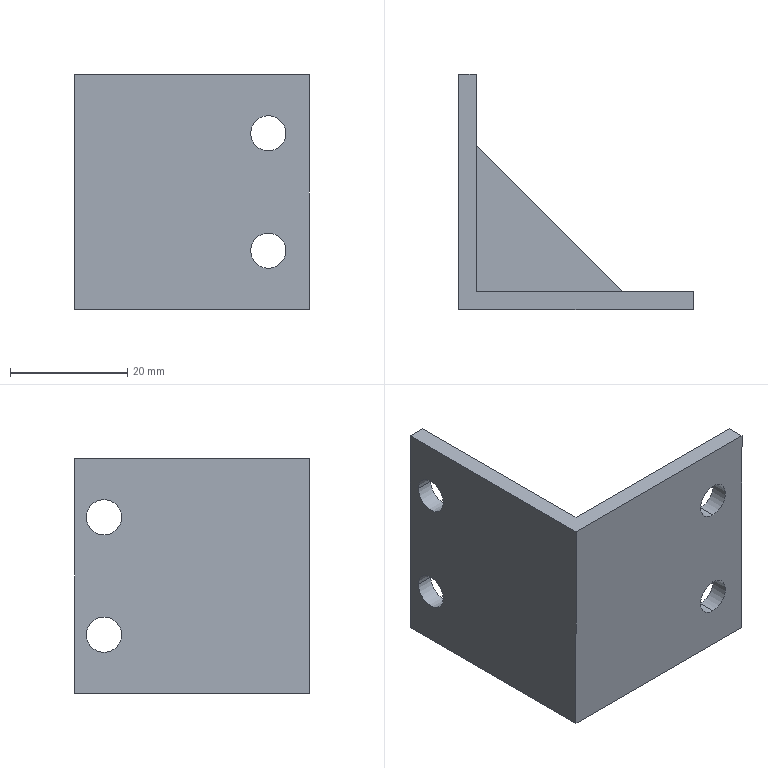Part | SolidWorks | features ICE 2, FlatPattern 1, Gusset 1, SMBaseFlange 1, SheetMetal 1 | 2 solids | 21 faces | box 40 x 40 x 40 mm | volume 10463 mm3 | plane 13 | cylinder 8 | commonest cylinder face diameters 6 x8
STEP:
#1=CARTESIAN_POINT('',(3.,28.,-17.5));
#2=VERTEX_POINT('',#1);
#3=CARTESIAN_POINT('',(28.,3.,-17.5));
#4=VERTEX_POINT('',#3);
#5=CARTESIAN_POINT('',(3.,28.,-17.5));
#6=DIRECTION('',(0.7071,-0.7071,0.));
#7=VECTOR('',#6,1000.);
#8=LINE('',#5,#7);
#9=EDGE_CURVE('',#2,#4,#8,.T.);
#10=ORIENTED_EDGE('',*,*,#9,.T.);
#11=CARTESIAN_POINT('',(28.,3.,-22.5));
#12=VERTEX_POINT('',#11);
#13=CARTESIAN_POINT('',(28.,3.,-22.5));
#14=DIRECTION('',(0.,0.,1.));
#15=VECTOR('',#14,1000.);
#16=LINE('',#13,#15);
#17=EDGE_CURVE('',#12,#4,#16,.T.);
#18=ORIENTED_EDGE('',*,*,#17,.F.);
#19=CARTESIAN_POINT('',(3.,28.,-22.5));
#20=VERTEX_POINT('',#19);
#21=CARTESIAN_POINT('',(3.,28.,-22.5));
#22=DIRECTION('',(0.7071,-0.7071,0.));
#23=VECTOR('',#22,1000.);
#24=LINE('',#21,#23);
#25=EDGE_CURVE('',#20,#12,#24,.T.);
#26=ORIENTED_EDGE('',*,*,#25,.F.);
#27=CARTESIAN_POINT('',(3.,28.,-22.5));
#28=DIRECTION('',(0.,0.,1.));
#29=VECTOR('',#28,1000.);
#30=LINE('',#27,#29);
#31=EDGE_CURVE('',#20,#2,#30,.T.);
#32=ORIENTED_EDGE('',*,*,#31,.T.);
#33=EDGE_LOOP('',(#10,#18,#26,#32));
#34=FACE_OUTER_BOUND('',#33,.T.);
#35=CARTESIAN_POINT('',(3.,28.,-22.5));
#36=DIRECTION('',(-0.7071,-0.7071,0.));
#37=DIRECTION('',(0.7071,-0.7071,0.));
#38=AXIS2_PLACEMENT_3D('',#35,#36,#37);
#39=PLANE('',#38);
#40=ADVANCED_FACE('',(#34),#39,.F.);
#41=CARTESIAN_POINT('',(3.,3.,-17.5));
#42=VERTEX_POINT('',#41);
#43=CARTESIAN_POINT('',(3.,3.,-17.5));
#44=DIRECTION('',(-1.,0.,0.));
#45=VECTOR('',#44,1000.);
#46=LINE('',#43,#45);
#47=EDGE_CURVE('',#4,#42,#46,.T.);
#48=ORIENTED_EDGE('',*,*,#47,.T.);
#49=CARTESIAN_POINT('',(3.,3.,-22.5));
#50=VERTEX_POINT('',#49);
#51=CARTESIAN_POINT('',(3.,3.,-22.5));
#52=DIRECTION('',(0.,0.,1.));
#53=VECTOR('',#52,1000.);
#54=LINE('',#51,#53);
#55=EDGE_CURVE('',#50,#42,#54,.T.);
#56=ORIENTED_EDGE('',*,*,#55,.F.);
#57=CARTESIAN_POINT('',(3.,3.,-22.5));
#58=DIRECTION('',(-1.,0.,0.));
#59=VECTOR('',#58,1000.);
#60=LINE('',#57,#59);
#61=EDGE_CURVE('',#12,#50,#60,.T.);
#62=ORIENTED_EDGE('',*,*,#61,.F.);
#63=ORIENTED_EDGE('',*,*,#17,.T.);
#64=EDGE_LOOP('',(#48,#56,#62,#63));
#65=FACE_OUTER_BOUND('',#64,.T.);
#66=CARTESIAN_POINT('',(3.,3.,-22.5));
#67=DIRECTION('',(0.,1.,0.));
#68=DIRECTION('',(0.,0.,1.));
#69=AXIS2_PLACEMENT_3D('',#66,#67,#68);
#70=PLANE('',#69);
#71=ADVANCED_FACE('',(#65),#70,.F.);
#72=CARTESIAN_POINT('',(3.,3.,-17.5));
#73=DIRECTION('',(0.,1.,0.));
#74=VECTOR('',#73,1000.);
#75=LINE('',#72,#74);
#76=EDGE_CURVE('',#42,#2,#75,.T.);
#77=ORIENTED_EDGE('',*,*,#76,.T.);
#78=ORIENTED_EDGE('',*,*,#31,.F.);
#79=CARTESIAN_POINT('',(3.,3.,-22.5));
#80=DIRECTION('',(0.,1.,0.));
#81=VECTOR('',#80,1000.);
#82=LINE('',#79,#81);
#83=EDGE_CURVE('',#50,#20,#82,.T.);
#84=ORIENTED_EDGE('',*,*,#83,.F.);
#85=ORIENTED_EDGE('',*,*,#55,.T.);
#86=EDGE_LOOP('',(#77,#78,#84,#85));
#87=FACE_OUTER_BOUND('',#86,.T.);
#88=CARTESIAN_POINT('',(3.,3.,-22.5));
#89=DIRECTION('',(1.,0.,0.));
#90=DIRECTION('',(0.,1.,0.));
#91=AXIS2_PLACEMENT_3D('',#88,#89,#90);
#92=PLANE('',#91);
#93=ADVANCED_FACE('',(#87),#92,.F.);
#94=ORIENTED_EDGE('',*,*,#25,.T.);
#95=ORIENTED_EDGE('',*,*,#61,.T.);
#96=ORIENTED_EDGE('',*,*,#83,.T.);
#97=EDGE_LOOP('',(#94,#95,#96));
#98=FACE_OUTER_BOUND('',#97,.T.);
#99=CARTESIAN_POINT('',(0.,0.,-22.5));
#100=DIRECTION('',(0.,0.,1.));
#101=DIRECTION('',(1.,0.,0.));
#102=AXIS2_PLACEMENT_3D('',#99,#100,#101);
#103=PLANE('',#102);
#104=ADVANCED_FACE('',(#98),#103,.F.);
#105=ORIENTED_EDGE('',*,*,#9,.F.);
#106=ORIENTED_EDGE('',*,*,#76,.F.);
#107=ORIENTED_EDGE('',*,*,#47,.F.);
#108=EDGE_LOOP('',(#105,#106,#107));
#109=FACE_OUTER_BOUND('',#108,.T.);
#110=CARTESIAN_POINT('',(0.,0.,-17.5));
#111=DIRECTION('',(0.,0.,1.));
#112=DIRECTION('',(1.,0.,0.));
#113=AXIS2_PLACEMENT_3D('',#110,#111,#112);
#114=PLANE('',#113);
#115=ADVANCED_FACE('',(#109),#114,.T.);
#116=CLOSED_SHELL('',(#40,#71,#93,#104,#115));
#117=MANIFOLD_SOLID_BREP('',#116);
#118=CARTESIAN_POINT('',(33.,0.,-27.));
#119=VERTEX_POINT('',#118);
#120=CARTESIAN_POINT('',(33.,0.,-33.));
#121=VERTEX_POINT('',#120);
#122=CARTESIAN_POINT('',(33.,0.,-30.));
#123=DIRECTION('',(0.,-1.,0.));
#124=DIRECTION('',(0.,0.,-1.));
#125=AXIS2_PLACEMENT_3D('',#122,#123,#124);
#126=CIRCLE('',#125,3.);
#127=EDGE_CURVE('',#119,#121,#126,.T.);
#128=ORIENTED_EDGE('',*,*,#127,.T.);
#129=CARTESIAN_POINT('',(33.,3.,-33.));
#130=VERTEX_POINT('',#129);
#131=CARTESIAN_POINT('',(33.,-7.,-33.));
#132=DIRECTION('',(0.,1.,0.));
#133=VECTOR('',#132,1000.);
#134=LINE('',#131,#133);
#135=EDGE_CURVE('',#121,#130,#134,.T.);
#136=ORIENTED_EDGE('',*,*,#135,.T.);
#137=CARTESIAN_POINT('',(33.,3.,-27.));
#138=VERTEX_POINT('',#137);
#139=CARTESIAN_POINT('',(33.,3.,-30.));
#140=DIRECTION('',(0.,1.,0.));
#141=DIRECTION('',(0.,0.,1.));
#142=AXIS2_PLACEMENT_3D('',#139,#140,#141);
#143=CIRCLE('',#142,3.);
#144=EDGE_CURVE('',#130,#138,#143,.T.);
#145=ORIENTED_EDGE('',*,*,#144,.T.);
#146=CARTESIAN_POINT('',(33.,-7.,-27.));
#147=DIRECTION('',(0.,1.,0.));
#148=VECTOR('',#147,1000.);
#149=LINE('',#146,#148);
#150=EDGE_CURVE('',#119,#138,#149,.T.);
#151=ORIENTED_EDGE('',*,*,#150,.F.);
#152=EDGE_LOOP('',(#128,#136,#145,#151));
#153=FACE_OUTER_BOUND('',#152,.T.);
#154=CARTESIAN_POINT('',(33.,-7.,-30.));
#155=DIRECTION('',(0.,1.,0.));
#156=DIRECTION('',(0.,0.,1.));
#157=AXIS2_PLACEMENT_3D('',#154,#155,#156);
#158=CYLINDRICAL_SURFACE('',#157,3.);
#159=ADVANCED_FACE('',(#153),#158,.F.);
#160=CARTESIAN_POINT('',(33.,0.,-7.));
#161=VERTEX_POINT('',#160);
#162=CARTESIAN_POINT('',(33.,0.,-13.));
#163=VERTEX_POINT('',#162);
#164=CARTESIAN_POINT('',(33.,0.,-10.));
#165=DIRECTION('',(0.,-1.,0.));
#166=DIRECTION('',(0.,0.,-1.));
#167=AXIS2_PLACEMENT_3D('',#164,#165,#166);
#168=CIRCLE('',#167,3.);
#169=EDGE_CURVE('',#161,#163,#168,.T.);
#170=ORIENTED_EDGE('',*,*,#169,.T.);
#171=CARTESIAN_POINT('',(33.,3.,-13.));
#172=VERTEX_POINT('',#171);
#173=CARTESIAN_POINT('',(33.,-7.,-13.));
#174=DIRECTION('',(0.,1.,0.));
#175=VECTOR('',#174,1000.);
#176=LINE('',#173,#175);
#177=EDGE_CURVE('',#163,#172,#176,.T.);
#178=ORIENTED_EDGE('',*,*,#177,.T.);
#179=CARTESIAN_POINT('',(33.,3.,-7.));
#180=VERTEX_POINT('',#179);
#181=CARTESIAN_POINT('',(33.,3.,-10.));
#182=DIRECTION('',(0.,1.,0.));
#183=DIRECTION('',(0.,0.,1.));
#184=AXIS2_PLACEMENT_3D('',#181,#182,#183);
#185=CIRCLE('',#184,3.);
#186=EDGE_CURVE('',#172,#180,#185,.T.);
#187=ORIENTED_EDGE('',*,*,#186,.T.);
#188=CARTESIAN_POINT('',(33.,-7.,-7.));
#189=DIRECTION('',(0.,1.,0.));
#190=VECTOR('',#189,1000.);
#191=LINE('',#188,#190);
#192=EDGE_CURVE('',#161,#180,#191,.T.);
#193=ORIENTED_EDGE('',*,*,#192,.F.);
#194=EDGE_LOOP('',(#170,#178,#187,#193));
#195=FACE_OUTER_BOUND('',#194,.T.);
#196=CARTESIAN_POINT('',(33.,-7.,-10.));
#197=DIRECTION('',(0.,1.,0.));
#198=DIRECTION('',(0.,0.,1.));
#199=AXIS2_PLACEMENT_3D('',#196,#197,#198);
#200=CYLINDRICAL_SURFACE('',#199,3.);
#201=ADVANCED_FACE('',(#195),#200,.F.);
#202=CARTESIAN_POINT('',(0.,38.,-10.));
#203=VERTEX_POINT('',#202);
#204=CARTESIAN_POINT('',(0.,32.,-10.));
#205=VERTEX_POINT('',#204);
#206=CARTESIAN_POINT('',(0.,35.,-10.));
#207=DIRECTION('',(-1.,0.,0.));
#208=DIRECTION('',(0.,0.,1.));
#209=AXIS2_PLACEMENT_3D('',#206,#207,#208);
#210=CIRCLE('',#209,3.);
#211=EDGE_CURVE('',#203,#205,#210,.T.);
#212=ORIENTED_EDGE('',*,*,#211,.T.);
#213=CARTESIAN_POINT('',(3.,32.,-10.));
#214=VERTEX_POINT('',#213);
#215=CARTESIAN_POINT('',(-7.,32.,-10.));
#216=DIRECTION('',(1.,0.,0.));
#217=VECTOR('',#216,1000.);
#218=LINE('',#215,#217);
#219=EDGE_CURVE('',#205,#214,#218,.T.);
#220=ORIENTED_EDGE('',*,*,#219,.T.);
#221=CARTESIAN_POINT('',(3.,38.,-10.));
#222=VERTEX_POINT('',#221);
#223=CARTESIAN_POINT('',(3.,35.,-10.));
#224=DIRECTION('',(1.,0.,0.));
#225=DIRECTION('',(0.,1.,0.));
#226=AXIS2_PLACEMENT_3D('',#223,#224,#225);
#227=CIRCLE('',#226,3.);
#228=EDGE_CURVE('',#214,#222,#227,.T.);
#229=ORIENTED_EDGE('',*,*,#228,.T.);
#230=CARTESIAN_POINT('',(-7.,38.,-10.));
#231=DIRECTION('',(1.,0.,0.));
#232=VECTOR('',#231,1000.);
#233=LINE('',#230,#232);
#234=EDGE_CURVE('',#203,#222,#233,.T.);
#235=ORIENTED_EDGE('',*,*,#234,.F.);
#236=EDGE_LOOP('',(#212,#220,#229,#235));
#237=FACE_OUTER_BOUND('',#236,.T.);
#238=CARTESIAN_POINT('',(-7.,35.,-10.));
#239=DIRECTION('',(1.,0.,0.));
#240=DIRECTION('',(0.,1.,0.));
#241=AXIS2_PLACEMENT_3D('',#238,#239,#240);
#242=CYLINDRICAL_SURFACE('',#241,3.);
#243=ADVANCED_FACE('',(#237),#242,.F.);
#244=CARTESIAN_POINT('',(0.,38.,-30.));
#245=VERTEX_POINT('',#244);
#246=CARTESIAN_POINT('',(0.,32.,-30.));
#247=VERTEX_POINT('',#246);
#248=CARTESIAN_POINT('',(0.,35.,-30.));
#249=DIRECTION('',(-1.,0.,0.));
#250=DIRECTION('',(0.,0.,1.));
#251=AXIS2_PLACEMENT_3D('',#248,#249,#250);
#252=CIRCLE('',#251,3.);
#253=EDGE_CURVE('',#245,#247,#252,.T.);
#254=ORIENTED_EDGE('',*,*,#253,.T.);
#255=CARTESIAN_POINT('',(3.,32.,-30.));
#256=VERTEX_POINT('',#255);
#257=CARTESIAN_POINT('',(-7.,32.,-30.));
#258=DIRECTION('',(1.,0.,0.));
#259=VECTOR('',#258,1000.);
#260=LINE('',#257,#259);
#261=EDGE_CURVE('',#247,#256,#260,.T.);
#262=ORIENTED_EDGE('',*,*,#261,.T.);
#263=CARTESIAN_POINT('',(3.,38.,-30.));
#264=VERTEX_POINT('',#263);
#265=CARTESIAN_POINT('',(3.,35.,-30.));
#266=DIRECTION('',(1.,0.,0.));
#267=DIRECTION('',(0.,1.,0.));
#268=AXIS2_PLACEMENT_3D('',#265,#266,#267);
#269=CIRCLE('',#268,3.);
#270=EDGE_CURVE('',#256,#264,#269,.T.);
#271=ORIENTED_EDGE('',*,*,#270,.T.);
#272=CARTESIAN_POINT('',(-7.,38.,-30.));
#273=DIRECTION('',(1.,0.,0.));
#274=VECTOR('',#273,1000.);
#275=LINE('',#272,#274);
#276=EDGE_CURVE('',#245,#264,#275,.T.);
#277=ORIENTED_EDGE('',*,*,#276,.F.);
#278=EDGE_LOOP('',(#254,#262,#271,#277));
#279=FACE_OUTER_BOUND('',#278,.T.);
#280=CARTESIAN_POINT('',(-7.,35.,-30.));
#281=DIRECTION('',(1.,0.,0.));
#282=DIRECTION('',(0.,1.,0.));
#283=AXIS2_PLACEMENT_3D('',#280,#281,#282);
#284=CYLINDRICAL_SURFACE('',#283,3.);
#285=ADVANCED_FACE('',(#279),#284,.F.);
#286=CARTESIAN_POINT('',(3.,40.,0.));
#287=VERTEX_POINT('',#286);
#288=CARTESIAN_POINT('',(0.,40.,0.));
#289=VERTEX_POINT('',#288);
#290=CARTESIAN_POINT('',(0.,40.,0.));
#291=DIRECTION('',(-1.,0.,0.));
#292=VECTOR('',#291,1000.);
#293=LINE('',#290,#292);
#294=EDGE_CURVE('',#287,#289,#293,.T.);
#295=ORIENTED_EDGE('',*,*,#294,.F.);
#296=CARTESIAN_POINT('',(3.,40.,-40.));
#297=VERTEX_POINT('',#296);
#298=CARTESIAN_POINT('',(3.,40.,-40.));
#299=DIRECTION('',(0.,0.,1.));
#300=VECTOR('',#299,1000.);
#301=LINE('',#298,#300);
#302=EDGE_CURVE('',#297,#287,#301,.T.);
#303=ORIENTED_EDGE('',*,*,#302,.F.);
#304=CARTESIAN_POINT('',(0.,40.,-40.));
#305=VERTEX_POINT('',#304);
#306=CARTESIAN_POINT('',(0.,40.,-40.));
#307=DIRECTION('',(-1.,0.,0.));
#308=VECTOR('',#307,1000.);
#309=LINE('',#306,#308);
#310=EDGE_CURVE('',#297,#305,#309,.T.);
#311=ORIENTED_EDGE('',*,*,#310,.T.);
#312=CARTESIAN_POINT('',(0.,40.,-40.));
#313=DIRECTION('',(0.,0.,1.));
#314=VECTOR('',#313,1000.);
#315=LINE('',#312,#314);
#316=EDGE_CURVE('',#305,#289,#315,.T.);
#317=ORIENTED_EDGE('',*,*,#316,.T.);
#318=EDGE_LOOP('',(#295,#303,#311,#317));
#319=FACE_OUTER_BOUND('',#318,.T.);
#320=CARTESIAN_POINT('',(0.,40.,-40.));
#321=DIRECTION('',(0.,1.,0.));
#322=DIRECTION('',(0.,0.,1.));
#323=AXIS2_PLACEMENT_3D('',#320,#321,#322);
#324=PLANE('',#323);
#325=ADVANCED_FACE('',(#319),#324,.T.);
#326=CARTESIAN_POINT('',(3.,35.,-10.));
#327=DIRECTION('',(1.,0.,0.));
#328=DIRECTION('',(0.,1.,0.));
#329=AXIS2_PLACEMENT_3D('',#326,#327,#328);
#330=CIRCLE('',#329,3.);
#331=EDGE_CURVE('',#222,#214,#330,.T.);
#332=ORIENTED_EDGE('',*,*,#331,.F.);
#333=ORIENTED_EDGE('',*,*,#228,.F.);
#334=EDGE_LOOP('',(#332,#333));
#335=FACE_BOUND('',#334,.T.);
#336=CARTESIAN_POINT('',(3.,35.,-30.));
#337=DIRECTION('',(1.,0.,0.));
#338=DIRECTION('',(0.,1.,0.));
#339=AXIS2_PLACEMENT_3D('',#336,#337,#338);
#340=CIRCLE('',#339,3.);
#341=EDGE_CURVE('',#264,#256,#340,.T.);
#342=ORIENTED_EDGE('',*,*,#341,.F.);
#343=ORIENTED_EDGE('',*,*,#270,.F.);
#344=EDGE_LOOP('',(#342,#343));
#345=FACE_BOUND('',#344,.T.);
#346=CARTESIAN_POINT('',(3.,3.,0.));
#347=VERTEX_POINT('',#346);
#348=CARTESIAN_POINT('',(3.,40.,0.));
#349=DIRECTION('',(0.,1.,0.));
#350=VECTOR('',#349,1000.);
#351=LINE('',#348,#350);
#352=EDGE_CURVE('',#347,#287,#351,.T.);
#353=ORIENTED_EDGE('',*,*,#352,.F.);
#354=CARTESIAN_POINT('',(3.,3.,-40.));
#355=VERTEX_POINT('',#354);
#356=CARTESIAN_POINT('',(3.,3.,-40.));
#357=DIRECTION('',(0.,0.,1.));
#358=VECTOR('',#357,1000.);
#359=LINE('',#356,#358);
#360=EDGE_CURVE('',#355,#347,#359,.T.);
#361=ORIENTED_EDGE('',*,*,#360,.F.);
#362=CARTESIAN_POINT('',(3.,40.,-40.));
#363=DIRECTION('',(0.,1.,0.));
#364=VECTOR('',#363,1000.);
#365=LINE('',#362,#364);
#366=EDGE_CURVE('',#355,#297,#365,.T.);
#367=ORIENTED_EDGE('',*,*,#366,.T.);
#368=ORIENTED_EDGE('',*,*,#302,.T.);
#369=EDGE_LOOP('',(#353,#361,#367,#368));
#370=FACE_OUTER_BOUND('',#369,.T.);
#371=CARTESIAN_POINT('',(3.,40.,-40.));
#372=DIRECTION('',(1.,0.,0.));
#373=DIRECTION('',(0.,1.,0.));
#374=AXIS2_PLACEMENT_3D('',#371,#372,#373);
#375=PLANE('',#374);
#376=ADVANCED_FACE('',(#335,#345,#370),#375,.T.);
#377=CARTESIAN_POINT('',(33.,3.,-30.));
#378=DIRECTION('',(0.,1.,0.));
#379=DIRECTION('',(0.,0.,1.));
#380=AXIS2_PLACEMENT_3D('',#377,#378,#379);
#381=CIRCLE('',#380,3.);
#382=EDGE_CURVE('',#138,#130,#381,.T.);
#383=ORIENTED_EDGE('',*,*,#382,.F.);
#384=ORIENTED_EDGE('',*,*,#144,.F.);
#385=EDGE_LOOP('',(#383,#384));
#386=FACE_BOUND('',#385,.T.);
#387=CARTESIAN_POINT('',(33.,3.,-10.));
#388=DIRECTION('',(0.,1.,0.));
#389=DIRECTION('',(0.,0.,1.));
#390=AXIS2_PLACEMENT_3D('',#387,#388,#389);
#391=CIRCLE('',#390,3.);
#392=EDGE_CURVE('',#180,#172,#391,.T.);
#393=ORIENTED_EDGE('',*,*,#392,.F.);
#394=ORIENTED_EDGE('',*,*,#186,.F.);
#395=EDGE_LOOP('',(#393,#394));
#396=FACE_BOUND('',#395,.T.);
#397=CARTESIAN_POINT('',(40.,3.,0.));
#398=VERTEX_POINT('',#397);
#399=CARTESIAN_POINT('',(3.,3.,0.));
#400=DIRECTION('',(-1.,0.,0.));
#401=VECTOR('',#400,1000.);
#402=LINE('',#399,#401);
#403=EDGE_CURVE('',#398,#347,#402,.T.);
#404=ORIENTED_EDGE('',*,*,#403,.F.);
#405=CARTESIAN_POINT('',(40.,3.,-40.));
#406=VERTEX_POINT('',#405);
#407=CARTESIAN_POINT('',(40.,3.,-40.));
#408=DIRECTION('',(0.,0.,1.));
#409=VECTOR('',#408,1000.);
#410=LINE('',#407,#409);
#411=EDGE_CURVE('',#406,#398,#410,.T.);
#412=ORIENTED_EDGE('',*,*,#411,.F.);
#413=CARTESIAN_POINT('',(3.,3.,-40.));
#414=DIRECTION('',(-1.,0.,0.));
#415=VECTOR('',#414,1000.);
#416=LINE('',#413,#415);
#417=EDGE_CURVE('',#406,#355,#416,.T.);
#418=ORIENTED_EDGE('',*,*,#417,.T.);
#419=ORIENTED_EDGE('',*,*,#360,.T.);
#420=EDGE_LOOP('',(#404,#412,#418,#419));
#421=FACE_OUTER_BOUND('',#420,.T.);
#422=CARTESIAN_POINT('',(3.,3.,-40.));
#423=DIRECTION('',(0.,1.,0.));
#424=DIRECTION('',(0.,0.,1.));
#425=AXIS2_PLACEMENT_3D('',#422,#423,#424);
#426=PLANE('',#425);
#427=ADVANCED_FACE('',(#386,#396,#421),#426,.T.);
#428=CARTESIAN_POINT('',(40.,0.,0.));
#429=VERTEX_POINT('',#428);
#430=CARTESIAN_POINT('',(40.,3.,0.));
#431=DIRECTION('',(0.,1.,0.));
#432=VECTOR('',#431,1000.);
#433=LINE('',#430,#432);
#434=EDGE_CURVE('',#429,#398,#433,.T.);
#435=ORIENTED_EDGE('',*,*,#434,.F.);
#436=CARTESIAN_POINT('',(40.,0.,-40.));
#437=VERTEX_POINT('',#436);
#438=CARTESIAN_POINT('',(40.,0.,-40.));
#439=DIRECTION('',(0.,0.,1.));
#440=VECTOR('',#439,1000.);
#441=LINE('',#438,#440);
#442=EDGE_CURVE('',#437,#429,#441,.T.);
#443=ORIENTED_EDGE('',*,*,#442,.F.);
#444=CARTESIAN_POINT('',(40.,3.,-40.));
#445=DIRECTION('',(0.,1.,0.));
#446=VECTOR('',#445,1000.);
#447=LINE('',#444,#446);
#448=EDGE_CURVE('',#437,#406,#447,.T.);
#449=ORIENTED_EDGE('',*,*,#448,.T.);
#450=ORIENTED_EDGE('',*,*,#411,.T.);
#451=EDGE_LOOP('',(#435,#443,#449,#450));
#452=FACE_OUTER_BOUND('',#451,.T.);
#453=CARTESIAN_POINT('',(40.,3.,-40.));
#454=DIRECTION('',(1.,0.,0.));
#455=DIRECTION('',(0.,0.,-1.));
#456=AXIS2_PLACEMENT_3D('',#453,#454,#455);
#457=PLANE('',#456);
#458=ADVANCED_FACE('',(#452),#457,.T.);
#459=ORIENTED_EDGE('',*,*,#127,.F.);
#460=CARTESIAN_POINT('',(33.,0.,-30.));
#461=DIRECTION('',(0.,-1.,0.));
#462=DIRECTION('',(0.,0.,-1.));
#463=AXIS2_PLACEMENT_3D('',#460,#461,#462);
#464=CIRCLE('',#463,3.);
#465=EDGE_CURVE('',#121,#119,#464,.T.);
#466=ORIENTED_EDGE('',*,*,#465,.F.);
#467=EDGE_LOOP('',(#459,#466));
#468=FACE_BOUND('',#467,.T.);
#469=ORIENTED_EDGE('',*,*,#169,.F.);
#470=CARTESIAN_POINT('',(33.,0.,-10.));
#471=DIRECTION('',(0.,-1.,0.));
#472=DIRECTION('',(0.,0.,-1.));
#473=AXIS2_PLACEMENT_3D('',#470,#471,#472);
#474=CIRCLE('',#473,3.);
#475=EDGE_CURVE('',#163,#161,#474,.T.);
#476=ORIENTED_EDGE('',*,*,#475,.F.);
#477=EDGE_LOOP('',(#469,#476));
#478=FACE_BOUND('',#477,.T.);
#479=CARTESIAN_POINT('',(0.,0.,0.));
#480=VERTEX_POINT('',#479);
#481=CARTESIAN_POINT('',(0.,0.,0.));
#482=DIRECTION('',(1.,0.,0.));
#483=VECTOR('',#482,1000.);
#484=LINE('',#481,#483);
#485=EDGE_CURVE('',#480,#429,#484,.T.);
#486=ORIENTED_EDGE('',*,*,#485,.F.);
#487=CARTESIAN_POINT('',(0.,0.,-40.));
#488=VERTEX_POINT('',#487);
#489=CARTESIAN_POINT('',(0.,0.,-40.));
#490=DIRECTION('',(0.,0.,1.));
#491=VECTOR('',#490,1000.);
#492=LINE('',#489,#491);
#493=EDGE_CURVE('',#488,#480,#492,.T.);
#494=ORIENTED_EDGE('',*,*,#493,.F.);
#495=CARTESIAN_POINT('',(0.,0.,-40.));
#496=DIRECTION('',(1.,0.,0.));
#497=VECTOR('',#496,1000.);
#498=LINE('',#495,#497);
#499=EDGE_CURVE('',#488,#437,#498,.T.);
#500=ORIENTED_EDGE('',*,*,#499,.T.);
#501=ORIENTED_EDGE('',*,*,#442,.T.);
#502=EDGE_LOOP('',(#486,#494,#500,#501));
#503=FACE_OUTER_BOUND('',#502,.T.);
#504=CARTESIAN_POINT('',(0.,0.,-40.));
#505=DIRECTION('',(0.,-1.,0.));
#506=DIRECTION('',(0.,0.,-1.));
#507=AXIS2_PLACEMENT_3D('',#504,#505,#506);
#508=PLANE('',#507);
#509=ADVANCED_FACE('',(#468,#478,#503),#508,.T.);
#510=ORIENTED_EDGE('',*,*,#211,.F.);
#511=CARTESIAN_POINT('',(0.,35.,-10.));
#512=DIRECTION('',(-1.,0.,0.));
#513=DIRECTION('',(0.,0.,1.));
#514=AXIS2_PLACEMENT_3D('',#511,#512,#513);
#515=CIRCLE('',#514,3.);
#516=EDGE_CURVE('',#205,#203,#515,.T.);
#517=ORIENTED_EDGE('',*,*,#516,.F.);
#518=EDGE_LOOP('',(#510,#517));
#519=FACE_BOUND('',#518,.T.);
#520=ORIENTED_EDGE('',*,*,#253,.F.);
#521=CARTESIAN_POINT('',(0.,35.,-30.));
#522=DIRECTION('',(-1.,0.,0.));
#523=DIRECTION('',(0.,0.,1.));
#524=AXIS2_PLACEMENT_3D('',#521,#522,#523);
#525=CIRCLE('',#524,3.);
#526=EDGE_CURVE('',#247,#245,#525,.T.);
#527=ORIENTED_EDGE('',*,*,#526,.F.);
#528=EDGE_LOOP('',(#520,#527));
#529=FACE_BOUND('',#528,.T.);
#530=CARTESIAN_POINT('',(0.,40.,0.));
#531=DIRECTION('',(0.,-1.,0.));
#532=VECTOR('',#531,1000.);
#533=LINE('',#530,#532);
#534=EDGE_CURVE('',#289,#480,#533,.T.);
#535=ORIENTED_EDGE('',*,*,#534,.F.);
#536=ORIENTED_EDGE('',*,*,#316,.F.);
#537=CARTESIAN_POINT('',(0.,40.,-40.));
#538=DIRECTION('',(0.,-1.,0.));
#539=VECTOR('',#538,1000.);
#540=LINE('',#537,#539);
#541=EDGE_CURVE('',#305,#488,#540,.T.);
#542=ORIENTED_EDGE('',*,*,#541,.T.);
#543=ORIENTED_EDGE('',*,*,#493,.T.);
#544=EDGE_LOOP('',(#535,#536,#542,#543));
#545=FACE_OUTER_BOUND('',#544,.T.);
#546=CARTESIAN_POINT('',(0.,40.,-40.));
#547=DIRECTION('',(-1.,0.,0.));
#548=DIRECTION('',(0.,0.,1.));
#549=AXIS2_PLACEMENT_3D('',#546,#547,#548);
#550=PLANE('',#549);
#551=ADVANCED_FACE('',(#519,#529,#545),#550,.T.);
#552=ORIENTED_EDGE('',*,*,#310,.F.);
#553=ORIENTED_EDGE('',*,*,#366,.F.);
#554=ORIENTED_EDGE('',*,*,#417,.F.);
#555=ORIENTED_EDGE('',*,*,#448,.F.);
#556=ORIENTED_EDGE('',*,*,#499,.F.);
#557=ORIENTED_EDGE('',*,*,#541,.F.);
#558=EDGE_LOOP('',(#552,#553,#554,#555,#556,#557));
#559=FACE_OUTER_BOUND('',#558,.T.);
#560=CARTESIAN_POINT('',(0.,0.,-40.));
#561=DIRECTION('',(0.,0.,-1.));
#562=DIRECTION('',(-1.,0.,0.));
#563=AXIS2_PLACEMENT_3D('',#560,#561,#562);
#564=PLANE('',#563);
#565=ADVANCED_FACE('',(#559),#564,.T.);
#566=ORIENTED_EDGE('',*,*,#294,.T.);
#567=ORIENTED_EDGE('',*,*,#534,.T.);
#568=ORIENTED_EDGE('',*,*,#485,.T.);
#569=ORIENTED_EDGE('',*,*,#434,.T.);
#570=ORIENTED_EDGE('',*,*,#403,.T.);
#571=ORIENTED_EDGE('',*,*,#352,.T.);
#572=EDGE_LOOP('',(#566,#567,#568,#569,#570,#571));
#573=FACE_OUTER_BOUND('',#572,.T.);
#574=CARTESIAN_POINT('',(0.,0.,0.));
#575=DIRECTION('',(0.,0.,-1.));
#576=DIRECTION('',(-1.,0.,0.));
#577=AXIS2_PLACEMENT_3D('',#574,#575,#576);
#578=PLANE('',#577);
#579=ADVANCED_FACE('',(#573),#578,.F.);
#580=ORIENTED_EDGE('',*,*,#261,.F.);
#581=ORIENTED_EDGE('',*,*,#526,.T.);
#582=ORIENTED_EDGE('',*,*,#276,.T.);
#583=ORIENTED_EDGE('',*,*,#341,.T.);
#584=EDGE_LOOP('',(#580,#581,#582,#583));
#585=FACE_OUTER_BOUND('',#584,.T.);
#586=CARTESIAN_POINT('',(-7.,35.,-30.));
#587=DIRECTION('',(1.,0.,0.));
#588=DIRECTION('',(0.,1.,0.));
#589=AXIS2_PLACEMENT_3D('',#586,#587,#588);
#590=CYLINDRICAL_SURFACE('',#589,3.);
#591=ADVANCED_FACE('',(#585),#590,.F.);
#592=ORIENTED_EDGE('',*,*,#219,.F.);
#593=ORIENTED_EDGE('',*,*,#516,.T.);
#594=ORIENTED_EDGE('',*,*,#234,.T.);
#595=ORIENTED_EDGE('',*,*,#331,.T.);
#596=EDGE_LOOP('',(#592,#593,#594,#595));
#597=FACE_OUTER_BOUND('',#596,.T.);
#598=CARTESIAN_POINT('',(-7.,35.,-10.));
#599=DIRECTION('',(1.,0.,0.));
#600=DIRECTION('',(0.,1.,0.));
#601=AXIS2_PLACEMENT_3D('',#598,#599,#600);
#602=CYLINDRICAL_SURFACE('',#601,3.);
#603=ADVANCED_FACE('',(#597),#602,.F.);
#604=ORIENTED_EDGE('',*,*,#177,.F.);
#605=ORIENTED_EDGE('',*,*,#475,.T.);
#606=ORIENTED_EDGE('',*,*,#192,.T.);
#607=ORIENTED_EDGE('',*,*,#392,.T.);
#608=EDGE_LOOP('',(#604,#605,#606,#607));
#609=FACE_OUTER_BOUND('',#608,.T.);
#610=CARTESIAN_POINT('',(33.,-7.,-10.));
#611=DIRECTION('',(0.,1.,0.));
#612=DIRECTION('',(0.,0.,1.));
#613=AXIS2_PLACEMENT_3D('',#610,#611,#612);
#614=CYLINDRICAL_SURFACE('',#613,3.);
#615=ADVANCED_FACE('',(#609),#614,.F.);
#616=ORIENTED_EDGE('',*,*,#135,.F.);
#617=ORIENTED_EDGE('',*,*,#465,.T.);
#618=ORIENTED_EDGE('',*,*,#150,.T.);
#619=ORIENTED_EDGE('',*,*,#382,.T.);
#620=EDGE_LOOP('',(#616,#617,#618,#619));
#621=FACE_OUTER_BOUND('',#620,.T.);
#622=CARTESIAN_POINT('',(33.,-7.,-30.));
#623=DIRECTION('',(0.,1.,0.));
#624=DIRECTION('',(0.,0.,1.));
#625=AXIS2_PLACEMENT_3D('',#622,#623,#624);
#626=CYLINDRICAL_SURFACE('',#625,3.);
#627=ADVANCED_FACE('',(#621),#626,.F.);
#628=CLOSED_SHELL('',(#159,#201,#243,#285,#325,#376,#427,#458,#509,#551,#565,#579,#591,#603,#615,#627));
#629=MANIFOLD_SOLID_BREP('',#628);
#630=CARTESIAN_POINT('',(0.,0.,0.));
#631=DIRECTION('',(0.,0.,1.));
#632=DIRECTION('',(1.,0.,0.));
#633=AXIS2_PLACEMENT_3D('',#630,#631,#632);
#634=(LENGTH_UNIT()NAMED_UNIT(*)SI_UNIT(.MILLI.,.METRE.));
#635=UNCERTAINTY_MEASURE_WITH_UNIT(LENGTH_MEASURE(0.00001),#634,'','');
#636=(NAMED_UNIT(*)PLANE_ANGLE_UNIT()SI_UNIT($,.RADIAN.));
#637=(NAMED_UNIT(*)SI_UNIT($,.STERADIAN.)SOLID_ANGLE_UNIT());
#638=(GEOMETRIC_REPRESENTATION_CONTEXT(3)GLOBAL_UNCERTAINTY_ASSIGNED_CONTEXT((#635))GLOBAL_UNIT_ASSIGNED_CONTEXT((#634,#636,#637))REPRESENTATION_CONTEXT('',''));
#639=ADVANCED_BREP_SHAPE_REPRESENTATION('',(#117,#629,#633),#638);